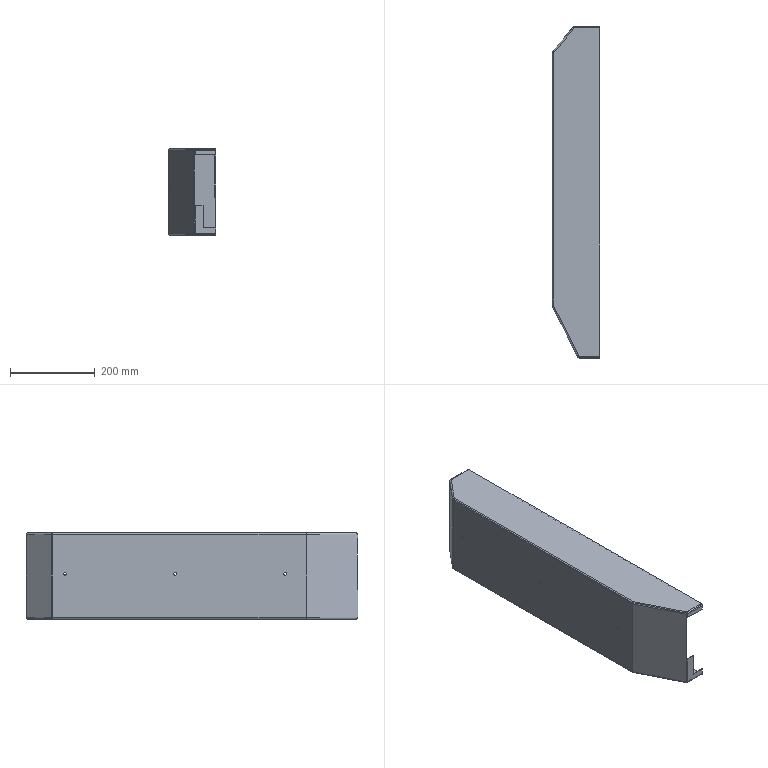Part | NX | features 5003_226_Cover 2 | 1 solid | 71 faces | box 112 x 784 x 204 mm | volume 699581 mm3 | plane 37 | cylinder 26 | sphere 8 | commonest cylinder face diameters 8 x14 6 x4 6.8 x3 7 x2 20 x2 4.134 x1